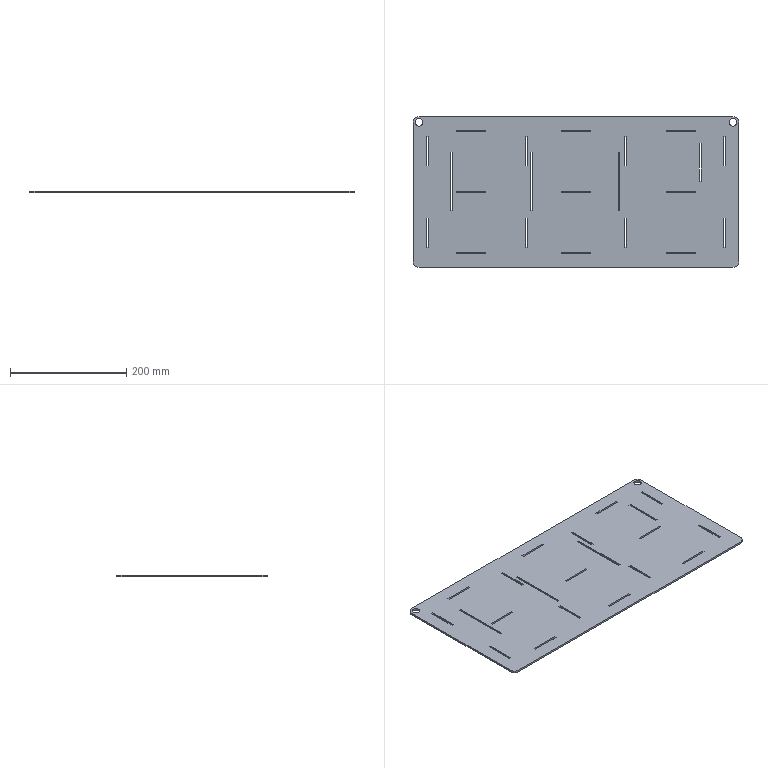Part | SolidWorks | features FlatPattern 1, SMBaseFlange 1, SheetMetal 1 | 1 solid | 98 faces | box 560 x 260 x 3.2 mm | volume 452354 mm3 | plane 90 | cylinder 8 | commonest cylinder face diameters 13 x4 20 x4